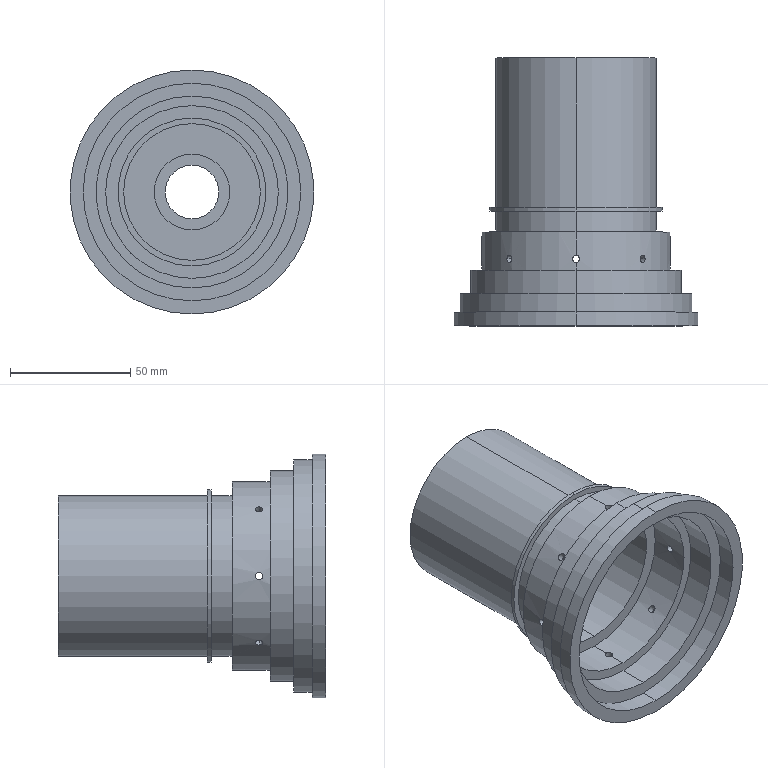Part | SolidWorks | features SavedExtBody 1 | 1 solid | 64 faces | box 101.384 x 111.36 x 101.384 mm | volume 137958 mm3 | cylinder 48 | plane 16 | commonest cylinder face diameters 3 x16 61.509 x4 66.617 x4 71.798 x4 22.352 x2 31.502 x2